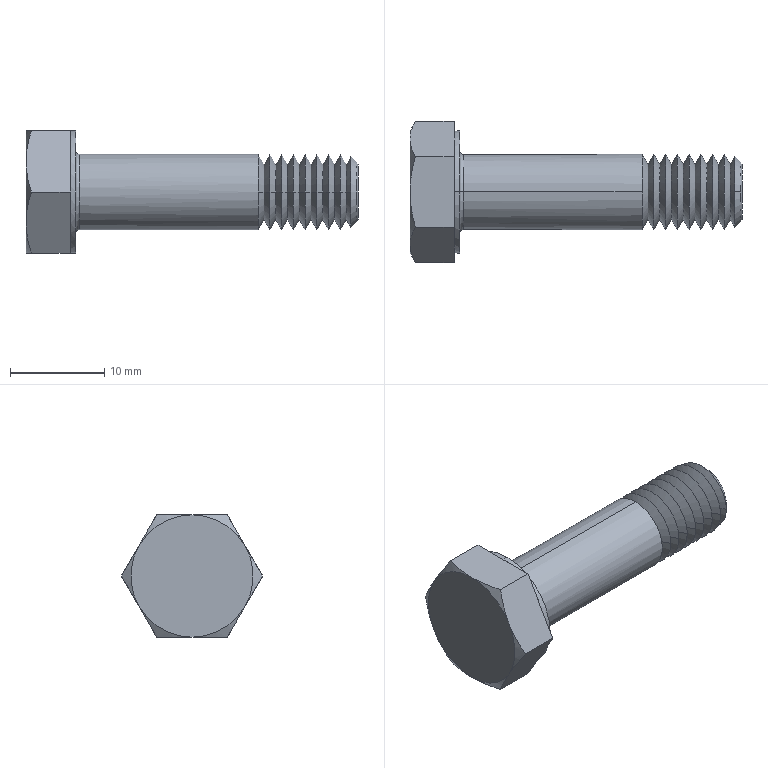Part | SolidWorks | features RevCut 4, Chamfer 1, Extrusion 1, Fillet 1, LPattern 1, Revolution 1 | 1 solid | 77 faces | box 35.3 x 15.011 x 13 mm | volume 2140 mm3 | cone 42 | cylinder 18 | plane 15 | torus 2 | commonest cylinder face diameters 8 x16 13 x2